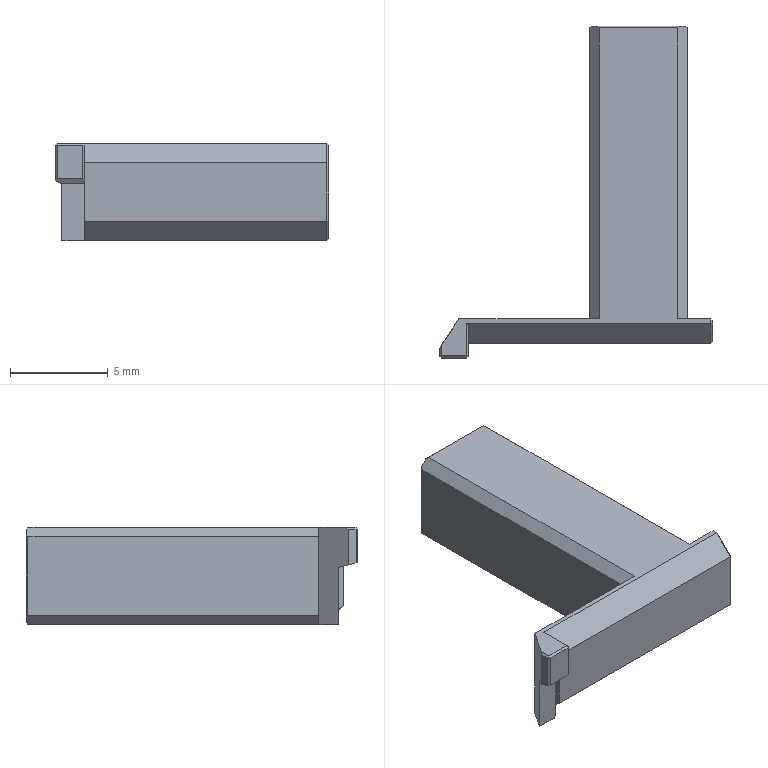Part | 1 solid | 45 faces | box 14 x 17 x 5 mm | volume 429.068 mm3 | plane 41 | cylinder 2 | cone 2 | commonest cylinder face diameters 1.6 x2
STEP:
#1=CARTESIAN_POINT('',(0.,9.8,-0.8));
#2=VERTEX_POINT('',#1);
#3=CARTESIAN_POINT('',(0.,9.8,0.8));
#4=VERTEX_POINT('',#3);
#5=CARTESIAN_POINT('',(0.,9.8,0.));
#6=DIRECTION('',(0.,1.,0.));
#7=DIRECTION('',(0.,0.,1.));
#8=AXIS2_PLACEMENT_3D('',#5,#6,#7);
#9=CIRCLE('',#8,0.8);
#10=EDGE_CURVE('',#2,#4,#9,.T.);
#11=ORIENTED_EDGE('',*,*,#10,.F.);
#12=CARTESIAN_POINT('',(0.,15.,-0.8));
#13=VERTEX_POINT('',#12);
#14=CARTESIAN_POINT('',(0.,15.,-0.8));
#15=DIRECTION('',(0.,1.,0.));
#16=VECTOR('',#15,1000.);
#17=LINE('',#14,#16);
#18=EDGE_CURVE('',#2,#13,#17,.T.);
#19=ORIENTED_EDGE('',*,*,#18,.T.);
#20=CARTESIAN_POINT('',(0.,15.,0.8));
#21=VERTEX_POINT('',#20);
#22=CARTESIAN_POINT('',(0.,15.,0.));
#23=DIRECTION('',(0.,1.,0.));
#24=DIRECTION('',(0.,0.,1.));
#25=AXIS2_PLACEMENT_3D('',#22,#23,#24);
#26=CIRCLE('',#25,0.8);
#27=EDGE_CURVE('',#13,#21,#26,.T.);
#28=ORIENTED_EDGE('',*,*,#27,.T.);
#29=CARTESIAN_POINT('',(0.,15.,0.8));
#30=DIRECTION('',(0.,1.,0.));
#31=VECTOR('',#30,1000.);
#32=LINE('',#29,#31);
#33=EDGE_CURVE('',#4,#21,#32,.T.);
#34=ORIENTED_EDGE('',*,*,#33,.F.);
#35=EDGE_LOOP('',(#11,#19,#28,#34));
#36=FACE_OUTER_BOUND('',#35,.T.);
#37=CARTESIAN_POINT('',(0.,15.,0.));
#38=DIRECTION('',(0.,1.,0.));
#39=DIRECTION('',(0.,0.,1.));
#40=AXIS2_PLACEMENT_3D('',#37,#38,#39);
#41=CYLINDRICAL_SURFACE('',#40,0.8);
#42=ADVANCED_FACE('',(#36),#41,.F.);
#43=CARTESIAN_POINT('',(0.,9.319,0.));
#44=VERTEX_POINT('',#43);
#45=CARTESIAN_POINT('',(0.,9.8,0.8));
#46=DIRECTION('',(0.,0.515,0.8572));
#47=VECTOR('',#46,1000.);
#48=LINE('',#45,#47);
#49=EDGE_CURVE('',#44,#4,#48,.T.);
#50=ORIENTED_EDGE('',*,*,#49,.F.);
#51=CARTESIAN_POINT('',(0.,9.8,-0.8));
#52=DIRECTION('',(0.,0.515,-0.8572));
#53=VECTOR('',#52,1000.);
#54=LINE('',#51,#53);
#55=EDGE_CURVE('',#44,#2,#54,.T.);
#56=ORIENTED_EDGE('',*,*,#55,.T.);
#57=ORIENTED_EDGE('',*,*,#10,.T.);
#58=EDGE_LOOP('',(#50,#56,#57));
#59=FACE_OUTER_BOUND('',#58,.T.);
#60=CARTESIAN_POINT('',(0.,9.8,0.));
#61=DIRECTION('',(0.,1.,0.));
#62=DIRECTION('',(0.,0.,1.));
#63=AXIS2_PLACEMENT_3D('',#60,#61,#62);
#64=CONICAL_SURFACE('',#63,0.8,1.03);
#65=ADVANCED_FACE('',(#59),#64,.F.);
#66=CARTESIAN_POINT('',(-8.7,-1.9,2.4));
#67=VERTEX_POINT('',#66);
#68=CARTESIAN_POINT('',(-8.7,-1.9,0.6751));
#69=VERTEX_POINT('',#68);
#70=CARTESIAN_POINT('',(-8.7,-1.9,-2.5));
#71=DIRECTION('',(0.,0.,-1.));
#72=VECTOR('',#71,1000.);
#73=LINE('',#70,#72);
#74=EDGE_CURVE('',#67,#69,#73,.T.);
#75=ORIENTED_EDGE('',*,*,#74,.T.);
#76=CARTESIAN_POINT('',(-8.7,-1.25,0.501));
#77=VERTEX_POINT('',#76);
#78=CARTESIAN_POINT('',(-8.7,-2.,0.7019));
#79=DIRECTION('',(0.,0.9659,-0.2588));
#80=VECTOR('',#79,1000.);
#81=LINE('',#78,#80);
#82=EDGE_CURVE('',#69,#77,#81,.T.);
#83=ORIENTED_EDGE('',*,*,#82,.T.);
#84=CARTESIAN_POINT('',(-8.7,-1.25,1.5));
#85=VERTEX_POINT('',#84);
#86=CARTESIAN_POINT('',(-8.7,-1.25,-2.5));
#87=DIRECTION('',(0.,0.,1.));
#88=VECTOR('',#87,1000.);
#89=LINE('',#86,#88);
#90=EDGE_CURVE('',#77,#85,#89,.T.);
#91=ORIENTED_EDGE('',*,*,#90,.T.);
#92=CARTESIAN_POINT('',(-8.7,-0.35,2.4));
#93=VERTEX_POINT('',#92);
#94=CARTESIAN_POINT('',(-8.7,-3.625,-0.875));
#95=DIRECTION('',(0.,0.7071,0.7071));
#96=VECTOR('',#95,1000.);
#97=LINE('',#94,#96);
#98=EDGE_CURVE('',#85,#93,#97,.T.);
#99=ORIENTED_EDGE('',*,*,#98,.T.);
#100=CARTESIAN_POINT('',(-8.7,-2.,2.4));
#101=DIRECTION('',(0.,-1.,0.));
#102=VECTOR('',#101,1000.);
#103=LINE('',#100,#102);
#104=EDGE_CURVE('',#93,#67,#103,.T.);
#105=ORIENTED_EDGE('',*,*,#104,.T.);
#106=EDGE_LOOP('',(#75,#83,#91,#99,#105));
#107=FACE_OUTER_BOUND('',#106,.T.);
#108=CARTESIAN_POINT('',(-8.7,-2.,-2.5));
#109=DIRECTION('',(-1.,0.,0.));
#110=DIRECTION('',(0.,0.,1.));
#111=AXIS2_PLACEMENT_3D('',#108,#109,#110);
#112=PLANE('',#111);
#113=ADVANCED_FACE('',(#107),#112,.F.);
#114=CARTESIAN_POINT('',(2.5,14.9,-2.));
#115=VERTEX_POINT('',#114);
#116=CARTESIAN_POINT('',(2.5,14.9,2.));
#117=VERTEX_POINT('',#116);
#118=CARTESIAN_POINT('',(2.5,14.9,2.5));
#119=DIRECTION('',(0.,0.,1.));
#120=VECTOR('',#119,1000.);
#121=LINE('',#118,#120);
#122=EDGE_CURVE('',#115,#117,#121,.T.);
#123=ORIENTED_EDGE('',*,*,#122,.T.);
#124=CARTESIAN_POINT('',(2.5,0.,2.));
#125=VERTEX_POINT('',#124);
#126=CARTESIAN_POINT('',(2.5,15.,2.));
#127=DIRECTION('',(0.,-1.,0.));
#128=VECTOR('',#127,1000.);
#129=LINE('',#126,#128);
#130=EDGE_CURVE('',#117,#125,#129,.T.);
#131=ORIENTED_EDGE('',*,*,#130,.T.);
#132=CARTESIAN_POINT('',(2.5,0.,-2.));
#133=VERTEX_POINT('',#132);
#134=CARTESIAN_POINT('',(2.5,0.,2.5));
#135=DIRECTION('',(0.,0.,-1.));
#136=VECTOR('',#135,1000.);
#137=LINE('',#134,#136);
#138=EDGE_CURVE('',#125,#133,#137,.T.);
#139=ORIENTED_EDGE('',*,*,#138,.T.);
#140=CARTESIAN_POINT('',(2.5,15.,-2.));
#141=DIRECTION('',(0.,1.,0.));
#142=VECTOR('',#141,1000.);
#143=LINE('',#140,#142);
#144=EDGE_CURVE('',#133,#115,#143,.T.);
#145=ORIENTED_EDGE('',*,*,#144,.T.);
#146=EDGE_LOOP('',(#123,#131,#139,#145));
#147=FACE_OUTER_BOUND('',#146,.T.);
#148=CARTESIAN_POINT('',(2.5,15.,2.5));
#149=DIRECTION('',(-1.,0.,0.));
#150=DIRECTION('',(0.,0.,1.));
#151=AXIS2_PLACEMENT_3D('',#148,#149,#150);
#152=PLANE('',#151);
#153=ADVANCED_FACE('',(#147),#152,.F.);
#154=CARTESIAN_POINT('',(-8.8,-0.25,-2.5));
#155=VERTEX_POINT('',#154);
#156=CARTESIAN_POINT('',(-8.8,-1.,-2.5));
#157=VERTEX_POINT('',#156);
#158=CARTESIAN_POINT('',(-8.8,15.,-2.5));
#159=DIRECTION('',(0.,-1.,0.));
#160=VECTOR('',#159,1000.);
#161=LINE('',#158,#160);
#162=EDGE_CURVE('',#155,#157,#161,.T.);
#163=ORIENTED_EDGE('',*,*,#162,.T.);
#164=CARTESIAN_POINT('',(-9.867,-1.,-2.5));
#165=VERTEX_POINT('',#164);
#166=CARTESIAN_POINT('',(-10.2,-1.,-2.5));
#167=DIRECTION('',(1.,0.,0.));
#168=VECTOR('',#167,1000.);
#169=LINE('',#166,#168);
#170=EDGE_CURVE('',#165,#157,#169,.T.);
#171=ORIENTED_EDGE('',*,*,#170,.F.);
#172=CARTESIAN_POINT('',(-9.2,0.,-2.5));
#173=VERTEX_POINT('',#172);
#174=CARTESIAN_POINT('',(-0.2154,13.477,-2.5));
#175=DIRECTION('',(0.5547,0.8321,0.));
#176=VECTOR('',#175,1000.);
#177=LINE('',#174,#176);
#178=EDGE_CURVE('',#165,#173,#177,.T.);
#179=ORIENTED_EDGE('',*,*,#178,.T.);
#180=CARTESIAN_POINT('',(-2.,0.,-2.5));
#181=VERTEX_POINT('',#180);
#182=CARTESIAN_POINT('',(3.8,0.,-2.5));
#183=DIRECTION('',(1.,0.,0.));
#184=VECTOR('',#183,1000.);
#185=LINE('',#182,#184);
#186=EDGE_CURVE('',#173,#181,#185,.T.);
#187=ORIENTED_EDGE('',*,*,#186,.T.);
#188=CARTESIAN_POINT('',(-2.,14.9,-2.5));
#189=VERTEX_POINT('',#188);
#190=CARTESIAN_POINT('',(-2.,15.,-2.5));
#191=DIRECTION('',(0.,1.,0.));
#192=VECTOR('',#191,1000.);
#193=LINE('',#190,#192);
#194=EDGE_CURVE('',#181,#189,#193,.T.);
#195=ORIENTED_EDGE('',*,*,#194,.T.);
#196=CARTESIAN_POINT('',(2.,14.9,-2.5));
#197=VERTEX_POINT('',#196);
#198=CARTESIAN_POINT('',(-2.5,14.9,-2.5));
#199=DIRECTION('',(1.,0.,0.));
#200=VECTOR('',#199,1000.);
#201=LINE('',#198,#200);
#202=EDGE_CURVE('',#189,#197,#201,.T.);
#203=ORIENTED_EDGE('',*,*,#202,.T.);
#204=CARTESIAN_POINT('',(2.,0.,-2.5));
#205=VERTEX_POINT('',#204);
#206=CARTESIAN_POINT('',(2.,15.,-2.5));
#207=DIRECTION('',(0.,-1.,0.));
#208=VECTOR('',#207,1000.);
#209=LINE('',#206,#208);
#210=EDGE_CURVE('',#197,#205,#209,.T.);
#211=ORIENTED_EDGE('',*,*,#210,.T.);
#212=CARTESIAN_POINT('',(3.7,0.,-2.5));
#213=VERTEX_POINT('',#212);
#214=CARTESIAN_POINT('',(3.8,0.,-2.5));
#215=DIRECTION('',(1.,0.,0.));
#216=VECTOR('',#215,1000.);
#217=LINE('',#214,#216);
#218=EDGE_CURVE('',#205,#213,#217,.T.);
#219=ORIENTED_EDGE('',*,*,#218,.T.);
#220=CARTESIAN_POINT('',(3.7,-0.25,-2.5));
#221=VERTEX_POINT('',#220);
#222=CARTESIAN_POINT('',(3.7,15.,-2.5));
#223=DIRECTION('',(0.,-1.,0.));
#224=VECTOR('',#223,1000.);
#225=LINE('',#222,#224);
#226=EDGE_CURVE('',#213,#221,#225,.T.);
#227=ORIENTED_EDGE('',*,*,#226,.T.);
#228=CARTESIAN_POINT('',(-2.5,-0.25,-2.5));
#229=DIRECTION('',(-1.,0.,0.));
#230=VECTOR('',#229,1000.);
#231=LINE('',#228,#230);
#232=EDGE_CURVE('',#221,#155,#231,.T.);
#233=ORIENTED_EDGE('',*,*,#232,.T.);
#234=EDGE_LOOP('',(#163,#171,#179,#187,#195,#203,#211,#219,#227,#233));
#235=FACE_OUTER_BOUND('',#234,.T.);
#236=CARTESIAN_POINT('',(-2.5,15.,-2.5));
#237=DIRECTION('',(0.,0.,1.));
#238=DIRECTION('',(1.,0.,0.));
#239=AXIS2_PLACEMENT_3D('',#236,#237,#238);
#240=PLANE('',#239);
#241=ADVANCED_FACE('',(#235),#240,.F.);
#242=CARTESIAN_POINT('',(-2.5,0.,-2.));
#243=VERTEX_POINT('',#242);
#244=CARTESIAN_POINT('',(-2.5,0.,2.));
#245=VERTEX_POINT('',#244);
#246=CARTESIAN_POINT('',(-2.5,0.,2.5));
#247=DIRECTION('',(0.,0.,1.));
#248=VECTOR('',#247,1000.);
#249=LINE('',#246,#248);
#250=EDGE_CURVE('',#243,#245,#249,.T.);
#251=ORIENTED_EDGE('',*,*,#250,.T.);
#252=CARTESIAN_POINT('',(-2.5,14.9,2.));
#253=VERTEX_POINT('',#252);
#254=CARTESIAN_POINT('',(-2.5,15.,2.));
#255=DIRECTION('',(0.,1.,0.));
#256=VECTOR('',#255,1000.);
#257=LINE('',#254,#256);
#258=EDGE_CURVE('',#245,#253,#257,.T.);
#259=ORIENTED_EDGE('',*,*,#258,.T.);
#260=CARTESIAN_POINT('',(-2.5,14.9,-2.));
#261=VERTEX_POINT('',#260);
#262=CARTESIAN_POINT('',(-2.5,14.9,2.5));
#263=DIRECTION('',(0.,0.,-1.));
#264=VECTOR('',#263,1000.);
#265=LINE('',#262,#264);
#266=EDGE_CURVE('',#253,#261,#265,.T.);
#267=ORIENTED_EDGE('',*,*,#266,.T.);
#268=CARTESIAN_POINT('',(-2.5,15.,-2.));
#269=DIRECTION('',(0.,-1.,0.));
#270=VECTOR('',#269,1000.);
#271=LINE('',#268,#270);
#272=EDGE_CURVE('',#261,#243,#271,.T.);
#273=ORIENTED_EDGE('',*,*,#272,.T.);
#274=EDGE_LOOP('',(#251,#259,#267,#273));
#275=FACE_OUTER_BOUND('',#274,.T.);
#276=CARTESIAN_POINT('',(-2.5,15.,2.5));
#277=DIRECTION('',(1.,0.,0.));
#278=DIRECTION('',(0.,0.,-1.));
#279=AXIS2_PLACEMENT_3D('',#276,#277,#278);
#280=PLANE('',#279);
#281=ADVANCED_FACE('',(#275),#280,.F.);
#282=CARTESIAN_POINT('',(-2.,0.,2.5));
#283=VERTEX_POINT('',#282);
#284=CARTESIAN_POINT('',(-9.2,0.,2.5));
#285=VERTEX_POINT('',#284);
#286=CARTESIAN_POINT('',(3.8,0.,2.5));
#287=DIRECTION('',(-1.,0.,0.));
#288=VECTOR('',#287,1000.);
#289=LINE('',#286,#288);
#290=EDGE_CURVE('',#283,#285,#289,.T.);
#291=ORIENTED_EDGE('',*,*,#290,.T.);
#292=CARTESIAN_POINT('',(-10.1,-1.35,2.5));
#293=VERTEX_POINT('',#292);
#294=CARTESIAN_POINT('',(-10.2,-1.5,2.5));
#295=DIRECTION('',(0.5547,0.8321,0.));
#296=VECTOR('',#295,1000.);
#297=LINE('',#294,#296);
#298=EDGE_CURVE('',#293,#285,#297,.T.);
#299=ORIENTED_EDGE('',*,*,#298,.F.);
#300=CARTESIAN_POINT('',(-10.1,-1.9,2.5));
#301=VERTEX_POINT('',#300);
#302=CARTESIAN_POINT('',(-10.1,15.,2.5));
#303=DIRECTION('',(0.,-1.,0.));
#304=VECTOR('',#303,1000.);
#305=LINE('',#302,#304);
#306=EDGE_CURVE('',#293,#301,#305,.T.);
#307=ORIENTED_EDGE('',*,*,#306,.T.);
#308=CARTESIAN_POINT('',(-8.8,-1.9,2.5));
#309=VERTEX_POINT('',#308);
#310=CARTESIAN_POINT('',(-2.5,-1.9,2.5));
#311=DIRECTION('',(1.,0.,0.));
#312=VECTOR('',#311,1000.);
#313=LINE('',#310,#312);
#314=EDGE_CURVE('',#301,#309,#313,.T.);
#315=ORIENTED_EDGE('',*,*,#314,.T.);
#316=CARTESIAN_POINT('',(-8.8,-0.25,2.5));
#317=VERTEX_POINT('',#316);
#318=CARTESIAN_POINT('',(-8.8,15.,2.5));
#319=DIRECTION('',(0.,1.,0.));
#320=VECTOR('',#319,1000.);
#321=LINE('',#318,#320);
#322=EDGE_CURVE('',#309,#317,#321,.T.);
#323=ORIENTED_EDGE('',*,*,#322,.T.);
#324=CARTESIAN_POINT('',(3.7,-0.25,2.5));
#325=VERTEX_POINT('',#324);
#326=CARTESIAN_POINT('',(-2.5,-0.25,2.5));
#327=DIRECTION('',(1.,0.,0.));
#328=VECTOR('',#327,1000.);
#329=LINE('',#326,#328);
#330=EDGE_CURVE('',#317,#325,#329,.T.);
#331=ORIENTED_EDGE('',*,*,#330,.T.);
#332=CARTESIAN_POINT('',(3.7,0.,2.5));
#333=VERTEX_POINT('',#332);
#334=CARTESIAN_POINT('',(3.7,15.,2.5));
#335=DIRECTION('',(0.,1.,0.));
#336=VECTOR('',#335,1000.);
#337=LINE('',#334,#336);
#338=EDGE_CURVE('',#325,#333,#337,.T.);
#339=ORIENTED_EDGE('',*,*,#338,.T.);
#340=CARTESIAN_POINT('',(2.,0.,2.5));
#341=VERTEX_POINT('',#340);
#342=CARTESIAN_POINT('',(3.8,0.,2.5));
#343=DIRECTION('',(-1.,0.,0.));
#344=VECTOR('',#343,1000.);
#345=LINE('',#342,#344);
#346=EDGE_CURVE('',#333,#341,#345,.T.);
#347=ORIENTED_EDGE('',*,*,#346,.T.);
#348=CARTESIAN_POINT('',(2.,14.9,2.5));
#349=VERTEX_POINT('',#348);
#350=CARTESIAN_POINT('',(2.,15.,2.5));
#351=DIRECTION('',(0.,1.,0.));
#352=VECTOR('',#351,1000.);
#353=LINE('',#350,#352);
#354=EDGE_CURVE('',#341,#349,#353,.T.);
#355=ORIENTED_EDGE('',*,*,#354,.T.);
#356=CARTESIAN_POINT('',(-2.,14.9,2.5));
#357=VERTEX_POINT('',#356);
#358=CARTESIAN_POINT('',(-2.5,14.9,2.5));
#359=DIRECTION('',(-1.,0.,0.));
#360=VECTOR('',#359,1000.);
#361=LINE('',#358,#360);
#362=EDGE_CURVE('',#349,#357,#361,.T.);
#363=ORIENTED_EDGE('',*,*,#362,.T.);
#364=CARTESIAN_POINT('',(-2.,15.,2.5));
#365=DIRECTION('',(0.,-1.,0.));
#366=VECTOR('',#365,1000.);
#367=LINE('',#364,#366);
#368=EDGE_CURVE('',#357,#283,#367,.T.);
#369=ORIENTED_EDGE('',*,*,#368,.T.);
#370=EDGE_LOOP('',(#291,#299,#307,#315,#323,#331,#339,#347,#355,#363,#369));
#371=FACE_OUTER_BOUND('',#370,.T.);
#372=CARTESIAN_POINT('',(-2.5,15.,2.5));
#373=DIRECTION('',(0.,0.,-1.));
#374=DIRECTION('',(-1.,0.,0.));
#375=AXIS2_PLACEMENT_3D('',#372,#373,#374);
#376=PLANE('',#375);
#377=ADVANCED_FACE('',(#371),#376,.F.);
#378=CARTESIAN_POINT('',(-2.4,15.,-2.1));
#379=VERTEX_POINT('',#378);
#380=CARTESIAN_POINT('',(-2.4,15.,2.1));
#381=VERTEX_POINT('',#380);
#382=CARTESIAN_POINT('',(-2.4,15.,0.));
#383=DIRECTION('',(0.,0.,1.));
#384=VECTOR('',#383,1000.);
#385=LINE('',#382,#384);
#386=EDGE_CURVE('',#379,#381,#385,.T.);
#387=ORIENTED_EDGE('',*,*,#386,.T.);
#388=CARTESIAN_POINT('',(-2.1,15.,2.4));
#389=VERTEX_POINT('',#388);
#390=CARTESIAN_POINT('',(-2.,15.,2.5));
#391=DIRECTION('',(0.7071,0.,0.7071));
#392=VECTOR('',#391,1000.);
#393=LINE('',#390,#392);
#394=EDGE_CURVE('',#381,#389,#393,.T.);
#395=ORIENTED_EDGE('',*,*,#394,.T.);
#396=CARTESIAN_POINT('',(2.1,15.,2.4));
#397=VERTEX_POINT('',#396);
#398=CARTESIAN_POINT('',(0.,15.,2.4));
#399=DIRECTION('',(1.,0.,0.));
#400=VECTOR('',#399,1000.);
#401=LINE('',#398,#400);
#402=EDGE_CURVE('',#389,#397,#401,.T.);
#403=ORIENTED_EDGE('',*,*,#402,.T.);
#404=CARTESIAN_POINT('',(2.4,15.,2.1));
#405=VERTEX_POINT('',#404);
#406=CARTESIAN_POINT('',(2.5,15.,2.));
#407=DIRECTION('',(0.7071,0.,-0.7071));
#408=VECTOR('',#407,1000.);
#409=LINE('',#406,#408);
#410=EDGE_CURVE('',#397,#405,#409,.T.);
#411=ORIENTED_EDGE('',*,*,#410,.T.);
#412=CARTESIAN_POINT('',(2.4,15.,-2.1));
#413=VERTEX_POINT('',#412);
#414=CARTESIAN_POINT('',(2.4,15.,0.));
#415=DIRECTION('',(0.,0.,-1.));
#416=VECTOR('',#415,1000.);
#417=LINE('',#414,#416);
#418=EDGE_CURVE('',#405,#413,#417,.T.);
#419=ORIENTED_EDGE('',*,*,#418,.T.);
#420=CARTESIAN_POINT('',(2.1,15.,-2.4));
#421=VERTEX_POINT('',#420);
#422=CARTESIAN_POINT('',(2.,15.,-2.5));
#423=DIRECTION('',(-0.7071,0.,-0.7071));
#424=VECTOR('',#423,1000.);
#425=LINE('',#422,#424);
#426=EDGE_CURVE('',#413,#421,#425,.T.);
#427=ORIENTED_EDGE('',*,*,#426,.T.);
#428=CARTESIAN_POINT('',(-2.1,15.,-2.4));
#429=VERTEX_POINT('',#428);
#430=CARTESIAN_POINT('',(0.,15.,-2.4));
#431=DIRECTION('',(-1.,0.,0.));
#432=VECTOR('',#431,1000.);
#433=LINE('',#430,#432);
#434=EDGE_CURVE('',#421,#429,#433,.T.);
#435=ORIENTED_EDGE('',*,*,#434,.T.);
#436=CARTESIAN_POINT('',(-2.5,15.,-2.));
#437=DIRECTION('',(-0.7071,0.,0.7071));
#438=VECTOR('',#437,1000.);
#439=LINE('',#436,#438);
#440=EDGE_CURVE('',#429,#379,#439,.T.);
#441=ORIENTED_EDGE('',*,*,#440,.T.);
#442=EDGE_LOOP('',(#387,#395,#403,#411,#419,#427,#435,#441));
#443=FACE_OUTER_BOUND('',#442,.T.);
#444=CARTESIAN_POINT('',(0.,15.,0.));
#445=DIRECTION('',(0.,1.,0.));
#446=DIRECTION('',(0.,0.,1.));
#447=AXIS2_PLACEMENT_3D('',#444,#445,#446);
#448=CIRCLE('',#447,0.8);
#449=EDGE_CURVE('',#21,#13,#448,.T.);
#450=ORIENTED_EDGE('',*,*,#449,.F.);
#451=ORIENTED_EDGE('',*,*,#27,.F.);
#452=EDGE_LOOP('',(#450,#451));
#453=FACE_BOUND('',#452,.T.);
#454=CARTESIAN_POINT('',(0.,15.,0.));
#455=DIRECTION('',(0.,-1.,0.));
#456=DIRECTION('',(0.,0.,-1.));
#457=AXIS2_PLACEMENT_3D('',#454,#455,#456);
#458=PLANE('',#457);
#459=ADVANCED_FACE('',(#443,#453),#458,.F.);
#460=ORIENTED_EDGE('',*,*,#55,.F.);
#461=ORIENTED_EDGE('',*,*,#49,.T.);
#462=CARTESIAN_POINT('',(0.,9.8,0.));
#463=DIRECTION('',(0.,1.,0.));
#464=DIRECTION('',(0.,0.,1.));
#465=AXIS2_PLACEMENT_3D('',#462,#463,#464);
#466=CIRCLE('',#465,0.8);
#467=EDGE_CURVE('',#4,#2,#466,.T.);
#468=ORIENTED_EDGE('',*,*,#467,.T.);
#469=EDGE_LOOP('',(#460,#461,#468));
#470=FACE_OUTER_BOUND('',#469,.T.);
#471=CARTESIAN_POINT('',(0.,9.8,0.));
#472=DIRECTION('',(0.,1.,0.));
#473=DIRECTION('',(0.,0.,1.));
#474=AXIS2_PLACEMENT_3D('',#471,#472,#473);
#475=CONICAL_SURFACE('',#474,0.8,1.03);
#476=ADVANCED_FACE('',(#470),#475,.F.);
#477=ORIENTED_EDGE('',*,*,#18,.F.);
#478=ORIENTED_EDGE('',*,*,#467,.F.);
#479=ORIENTED_EDGE('',*,*,#33,.T.);
#480=ORIENTED_EDGE('',*,*,#449,.T.);
#481=EDGE_LOOP('',(#477,#478,#479,#480));
#482=FACE_OUTER_BOUND('',#481,.T.);
#483=CARTESIAN_POINT('',(0.,15.,0.));
#484=DIRECTION('',(0.,1.,0.));
#485=DIRECTION('',(0.,0.,1.));
#486=AXIS2_PLACEMENT_3D('',#483,#484,#485);
#487=CYLINDRICAL_SURFACE('',#486,0.8);
#488=ADVANCED_FACE('',(#482),#487,.F.);
#489=ORIENTED_EDGE('',*,*,#346,.F.);
#490=CARTESIAN_POINT('',(3.7,0.,-2.5));
#491=DIRECTION('',(0.,0.,-1.));
#492=VECTOR('',#491,1000.);
#493=LINE('',#490,#492);
#494=EDGE_CURVE('',#333,#213,#493,.T.);
#495=ORIENTED_EDGE('',*,*,#494,.T.);
#496=ORIENTED_EDGE('',*,*,#218,.F.);
#497=CARTESIAN_POINT('',(2.,0.,-2.5));
#498=DIRECTION('',(0.7071,0.,0.7071));
#499=VECTOR('',#498,1000.);
#500=LINE('',#497,#499);
#501=EDGE_CURVE('',#205,#133,#500,.T.);
#502=ORIENTED_EDGE('',*,*,#501,.T.);
#503=ORIENTED_EDGE('',*,*,#138,.F.);
#504=CARTESIAN_POINT('',(2.5,0.,2.));
#505=DIRECTION('',(-0.7071,0.,0.7071));
#506=VECTOR('',#505,1000.);
#507=LINE('',#504,#506);
#508=EDGE_CURVE('',#125,#341,#507,.T.);
#509=ORIENTED_EDGE('',*,*,#508,.T.);
#510=EDGE_LOOP('',(#489,#495,#496,#502,#503,#509));
#511=FACE_OUTER_BOUND('',#510,.T.);
#512=CARTESIAN_POINT('',(0.,0.,0.));
#513=DIRECTION('',(0.,1.,0.));
#514=DIRECTION('',(0.,0.,1.));
#515=AXIS2_PLACEMENT_3D('',#512,#513,#514);
#516=PLANE('',#515);
#517=ADVANCED_FACE('',(#511),#516,.T.);
#518=CARTESIAN_POINT('',(-9.2,0.,-7.5));
#519=DIRECTION('',(0.,0.,1.));
#520=VECTOR('',#519,1000.);
#521=LINE('',#518,#520);
#522=EDGE_CURVE('',#173,#285,#521,.T.);
#523=ORIENTED_EDGE('',*,*,#522,.T.);
#524=ORIENTED_EDGE('',*,*,#290,.F.);
#525=CARTESIAN_POINT('',(-2.,0.,2.5));
#526=DIRECTION('',(-0.7071,0.,-0.7071));
#527=VECTOR('',#526,1000.);
#528=LINE('',#525,#527);
#529=EDGE_CURVE('',#283,#245,#528,.T.);
#530=ORIENTED_EDGE('',*,*,#529,.T.);
#531=ORIENTED_EDGE('',*,*,#250,.F.);
#532=CARTESIAN_POINT('',(-2.5,0.,-2.));
#533=DIRECTION('',(0.7071,0.,-0.7071));
#534=VECTOR('',#533,1000.);
#535=LINE('',#532,#534);
#536=EDGE_CURVE('',#243,#181,#535,.T.);
#537=ORIENTED_EDGE('',*,*,#536,.T.);
#538=ORIENTED_EDGE('',*,*,#186,.F.);
#539=EDGE_LOOP('',(#523,#524,#530,#531,#537,#538));
#540=FACE_OUTER_BOUND('',#539,.T.);
#541=CARTESIAN_POINT('',(0.,0.,0.));
#542=DIRECTION('',(0.,1.,0.));
#543=DIRECTION('',(0.,0.,1.));
#544=AXIS2_PLACEMENT_3D('',#541,#542,#543);
#545=PLANE('',#544);
#546=ADVANCED_FACE('',(#540),#545,.T.);
#547=CARTESIAN_POINT('',(3.8,-0.1,2.4));
#548=VERTEX_POINT('',#547);
#549=CARTESIAN_POINT('',(3.8,-0.2086,2.4));
#550=VERTEX_POINT('',#549);
#551=CARTESIAN_POINT('',(3.8,-2.,2.4));
#552=DIRECTION('',(0.,-1.,0.));
#553=VECTOR('',#552,1000.);
#554=LINE('',#551,#553);
#555=EDGE_CURVE('',#548,#550,#554,.T.);
#556=ORIENTED_EDGE('',*,*,#555,.T.);
#557=CARTESIAN_POINT('',(3.8,-1.15,1.459));
#558=VERTEX_POINT('',#557);
#559=CARTESIAN_POINT('',(3.8,-1.179,1.429));
#560=DIRECTION('',(0.,-0.7071,-0.7071));
#561=VECTOR('',#560,1000.);
#562=LINE('',#559,#561);
#563=EDGE_CURVE('',#550,#558,#562,.T.);
#564=ORIENTED_EDGE('',*,*,#563,.T.);
#565=CARTESIAN_POINT('',(3.8,-1.15,-1.459));
#566=VERTEX_POINT('',#565);
#567=CARTESIAN_POINT('',(3.8,-1.15,2.5));
#568=DIRECTION('',(0.,0.,-1.));
#569=VECTOR('',#568,1000.);
#570=LINE('',#567,#569);
#571=EDGE_CURVE('',#558,#566,#570,.T.);
#572=ORIENTED_EDGE('',*,*,#571,.T.);
#573=CARTESIAN_POINT('',(3.8,-0.2086,-2.4));
#574=VERTEX_POINT('',#573);
#575=CARTESIAN_POINT('',(3.8,-0.1793,-2.429));
#576=DIRECTION('',(0.,0.7071,-0.7071));
#577=VECTOR('',#576,1000.);
#578=LINE('',#575,#577);
#579=EDGE_CURVE('',#566,#574,#578,.T.);
#580=ORIENTED_EDGE('',*,*,#579,.T.);
#581=CARTESIAN_POINT('',(3.8,-0.1,-2.4));
#582=VERTEX_POINT('',#581);
#583=CARTESIAN_POINT('',(3.8,-2.,-2.4));
#584=DIRECTION('',(0.,1.,0.));
#585=VECTOR('',#584,1000.);
#586=LINE('',#583,#585);
#587=EDGE_CURVE('',#574,#582,#586,.T.);
#588=ORIENTED_EDGE('',*,*,#587,.T.);
#589=CARTESIAN_POINT('',(3.8,-0.1,2.5));
#590=DIRECTION('',(0.,0.,1.));
#591=VECTOR('',#590,1000.);
#592=LINE('',#589,#591);
#593=EDGE_CURVE('',#582,#548,#592,.T.);
#594=ORIENTED_EDGE('',*,*,#593,.T.);
#595=EDGE_LOOP('',(#556,#564,#572,#580,#588,#594));
#596=FACE_OUTER_BOUND('',#595,.T.);
#597=CARTESIAN_POINT('',(3.8,-2.,2.5));
#598=DIRECTION('',(-1.,0.,0.));
#599=DIRECTION('',(0.,0.,1.));
#600=AXIS2_PLACEMENT_3D('',#597,#598,#599);
#601=PLANE('',#600);
#602=ADVANCED_FACE('',(#596),#601,.F.);
#603=CARTESIAN_POINT('',(-10.2,-1.5,0.5679));
#604=VERTEX_POINT('',#603);
#605=CARTESIAN_POINT('',(-10.2,-1.5,2.4));
#606=VERTEX_POINT('',#605);
#607=CARTESIAN_POINT('',(-10.2,-1.5,-7.5));
#608=DIRECTION('',(0.,0.,1.));
#609=VECTOR('',#608,1000.);
#610=LINE('',#607,#609);
#611=EDGE_CURVE('',#604,#606,#610,.T.);
#612=ORIENTED_EDGE('',*,*,#611,.F.);
#613=CARTESIAN_POINT('',(-10.2,-1.9,0.6751));
#614=VERTEX_POINT('',#613);
#615=CARTESIAN_POINT('',(-10.2,-2.,0.7019));
#616=DIRECTION('',(0.,-0.9659,0.2588));
#617=VECTOR('',#616,1000.);
#618=LINE('',#615,#617);
#619=EDGE_CURVE('',#604,#614,#618,.T.);
#620=ORIENTED_EDGE('',*,*,#619,.T.);
#621=CARTESIAN_POINT('',(-10.2,-1.9,2.4));
#622=VERTEX_POINT('',#621);
#623=CARTESIAN_POINT('',(-10.2,-1.9,2.5));
#624=DIRECTION('',(0.,0.,1.));
#625=VECTOR('',#624,1000.);
#626=LINE('',#623,#625);
#627=EDGE_CURVE('',#614,#622,#626,.T.);
#628=ORIENTED_EDGE('',*,*,#627,.T.);
#629=CARTESIAN_POINT('',(-10.2,-2.,2.4));
#630=DIRECTION('',(0.,1.,0.));
#631=VECTOR('',#630,1000.);
#632=LINE('',#629,#631);
#633=EDGE_CURVE('',#622,#606,#632,.T.);
#634=ORIENTED_EDGE('',*,*,#633,.T.);
#635=EDGE_LOOP('',(#612,#620,#628,#634));
#636=FACE_OUTER_BOUND('',#635,.T.);
#637=CARTESIAN_POINT('',(-10.2,-2.,2.5));
#638=DIRECTION('',(1.,0.,0.));
#639=DIRECTION('',(0.,0.,-1.));
#640=AXIS2_PLACEMENT_3D('',#637,#638,#639);
#641=PLANE('',#640);
#642=ADVANCED_FACE('',(#636),#641,.F.);
#643=CARTESIAN_POINT('',(-10.1,-2.,2.4));
#644=VERTEX_POINT('',#643);
#645=CARTESIAN_POINT('',(-10.1,-2.,0.7019));
#646=VERTEX_POINT('',#645);
#647=CARTESIAN_POINT('',(-10.1,-2.,0.));
#648=DIRECTION('',(0.,0.,-1.));
#649=VECTOR('',#648,1000.);
#650=LINE('',#647,#649);
#651=EDGE_CURVE('',#644,#646,#650,.T.);
#652=ORIENTED_EDGE('',*,*,#651,.T.);
#653=CARTESIAN_POINT('',(-8.8,-2.,0.7019));
#654=VERTEX_POINT('',#653);
#655=CARTESIAN_POINT('',(0.,-2.,0.7019));
#656=DIRECTION('',(1.,0.,0.));
#657=VECTOR('',#656,1000.);
#658=LINE('',#655,#657);
#659=EDGE_CURVE('',#646,#654,#658,.T.);
#660=ORIENTED_EDGE('',*,*,#659,.T.);
#661=CARTESIAN_POINT('',(-8.8,-2.,2.4));
#662=VERTEX_POINT('',#661);
#663=CARTESIAN_POINT('',(-8.8,-2.,0.));
#664=DIRECTION('',(0.,0.,1.));
#665=VECTOR('',#664,1000.);
#666=LINE('',#663,#665);
#667=EDGE_CURVE('',#654,#662,#666,.T.);
#668=ORIENTED_EDGE('',*,*,#667,.T.);
#669=CARTESIAN_POINT('',(0.,-2.,2.4));
#670=DIRECTION('',(-1.,0.,0.));
#671=VECTOR('',#670,1000.);
#672=LINE('',#669,#671);
#673=EDGE_CURVE('',#662,#644,#672,.T.);
#674=ORIENTED_EDGE('',*,*,#673,.T.);
#675=EDGE_LOOP('',(#652,#660,#668,#674));
#676=FACE_OUTER_BOUND('',#675,.T.);
#677=CARTESIAN_POINT('',(0.,-2.,0.));
#678=DIRECTION('',(0.,1.,0.));
#679=DIRECTION('',(0.,0.,1.));
#680=AXIS2_PLACEMENT_3D('',#677,#678,#679);
#681=PLANE('',#680);
#682=ADVANCED_FACE('',(#676),#681,.F.);
#683=CARTESIAN_POINT('',(-8.7,-0.35,-2.4));
#684=VERTEX_POINT('',#683);
#685=CARTESIAN_POINT('',(-8.7,-1.,-1.75));
#686=VERTEX_POINT('',#685);
#687=CARTESIAN_POINT('',(-8.7,-1.125,-1.625));
#688=DIRECTION('',(0.,-0.7071,0.7071));
#689=VECTOR('',#688,1000.);
#690=LINE('',#687,#689);
#691=EDGE_CURVE('',#684,#686,#690,.T.);
#692=ORIENTED_EDGE('',*,*,#691,.T.);
#693=CARTESIAN_POINT('',(-8.7,-1.,-2.4));
#694=VERTEX_POINT('',#693);
#695=CARTESIAN_POINT('',(-8.7,-1.,0.3));
#696=DIRECTION('',(0.,0.,1.));
#697=VECTOR('',#696,1000.);
#698=LINE('',#695,#697);
#699=EDGE_CURVE('',#694,#686,#698,.T.);
#700=ORIENTED_EDGE('',*,*,#699,.F.);
#701=CARTESIAN_POINT('',(-8.7,-2.,-2.4));
#702=DIRECTION('',(0.,1.,0.));
#703=VECTOR('',#702,1000.);
#704=LINE('',#701,#703);
#705=EDGE_CURVE('',#694,#684,#704,.T.);
#706=ORIENTED_EDGE('',*,*,#705,.T.);
#707=EDGE_LOOP('',(#692,#700,#706));
#708=FACE_OUTER_BOUND('',#707,.T.);
#709=CARTESIAN_POINT('',(-8.7,-2.,-2.5));
#710=DIRECTION('',(-1.,0.,0.));
#711=DIRECTION('',(0.,0.,1.));
#712=AXIS2_PLACEMENT_3D('',#709,#710,#711);
#713=PLANE('',#712);
#714=ADVANCED_FACE('',(#708),#713,.F.);
#715=CARTESIAN_POINT('',(-8.7,-1.25,-1.5));
#716=VERTEX_POINT('',#715);
#717=CARTESIAN_POINT('',(3.7,-1.25,-1.5));
#718=VERTEX_POINT('',#717);
#719=CARTESIAN_POINT('',(3.8,-1.25,-1.5));
#720=DIRECTION('',(1.,0.,0.));
#721=VECTOR('',#720,1000.);
#722=LINE('',#719,#721);
#723=EDGE_CURVE('',#716,#718,#722,.T.);
#724=ORIENTED_EDGE('',*,*,#723,.T.);
#725=CARTESIAN_POINT('',(3.7,-1.25,1.5));
#726=VERTEX_POINT('',#725);
#727=CARTESIAN_POINT('',(3.7,-1.25,-2.5));
#728=DIRECTION('',(0.,0.,1.));
#729=VECTOR('',#728,1000.);
#730=LINE('',#727,#729);
#731=EDGE_CURVE('',#718,#726,#730,.T.);
#732=ORIENTED_EDGE('',*,*,#731,.T.);
#733=CARTESIAN_POINT('',(3.8,-1.25,1.5));
#734=DIRECTION('',(-1.,0.,0.));
#735=VECTOR('',#734,1000.);
#736=LINE('',#733,#735);
#737=EDGE_CURVE('',#726,#85,#736,.T.);
#738=ORIENTED_EDGE('',*,*,#737,.T.);
#739=ORIENTED_EDGE('',*,*,#90,.F.);
#740=CARTESIAN_POINT('',(-8.7,-1.25,-2.5));
#741=DIRECTION('',(0.,0.,1.));
#742=VECTOR('',#741,1000.);
#743=LINE('',#740,#742);
#744=EDGE_CURVE('',#716,#77,#743,.T.);
#745=ORIENTED_EDGE('',*,*,#744,.F.);
#746=EDGE_LOOP('',(#724,#732,#738,#739,#745));
#747=FACE_OUTER_BOUND('',#746,.T.);
#748=CARTESIAN_POINT('',(3.8,-1.25,-2.5));
#749=DIRECTION('',(0.,1.,0.));
#750=DIRECTION('',(-1.,0.,0.));
#751=AXIS2_PLACEMENT_3D('',#748,#749,#750);
#752=PLANE('',#751);
#753=ADVANCED_FACE('',(#747),#752,.F.);
#754=ORIENTED_EDGE('',*,*,#232,.F.);
#755=CARTESIAN_POINT('',(3.7,-1.25,-1.5));
#756=DIRECTION('',(0.,-0.7071,0.7071));
#757=VECTOR('',#756,1000.);
#758=LINE('',#755,#757);
#759=EDGE_CURVE('',#221,#718,#758,.T.);
#760=ORIENTED_EDGE('',*,*,#759,.T.);
#761=ORIENTED_EDGE('',*,*,#723,.F.);
#762=CARTESIAN_POINT('',(-8.7,-0.25,-2.5));
#763=DIRECTION('',(0.,0.7071,-0.7071));
#764=VECTOR('',#763,1000.);
#765=LINE('',#762,#764);
#766=EDGE_CURVE('',#716,#686,#765,.T.);
#767=ORIENTED_EDGE('',*,*,#766,.T.);
#768=ORIENTED_EDGE('',*,*,#691,.F.);
#769=CARTESIAN_POINT('',(-13.883,4.833,-7.583));
#770=DIRECTION('',(-0.5774,0.5774,-0.5774));
#771=VECTOR('',#770,1000.);
#772=LINE('',#769,#771);
#773=EDGE_CURVE('',#684,#155,#772,.T.);
#774=ORIENTED_EDGE('',*,*,#773,.T.);
#775=EDGE_LOOP('',(#754,#760,#761,#767,#768,#774));
#776=FACE_OUTER_BOUND('',#775,.T.);
#777=CARTESIAN_POINT('',(-2.5,-0.25,-2.5));
#778=DIRECTION('',(0.,0.7071,0.7071));
#779=DIRECTION('',(-1.,0.,0.));
#780=AXIS2_PLACEMENT_3D('',#777,#778,#779);
#781=PLANE('',#780);
#782=ADVANCED_FACE('',(#776),#781,.F.);
#783=ORIENTED_EDGE('',*,*,#737,.F.);
#784=CARTESIAN_POINT('',(3.7,-0.25,2.5));
#785=DIRECTION('',(0.,0.7071,0.7071));
#786=VECTOR('',#785,1000.);
#787=LINE('',#784,#786);
#788=EDGE_CURVE('',#726,#325,#787,.T.);
#789=ORIENTED_EDGE('',*,*,#788,.T.);
#790=ORIENTED_EDGE('',*,*,#330,.F.);
#791=CARTESIAN_POINT('',(-8.15,-0.9,1.85));
#792=DIRECTION('',(0.5774,-0.5774,-0.5774));
#793=VECTOR('',#792,1000.);
#794=LINE('',#791,#793);
#795=EDGE_CURVE('',#317,#93,#794,.T.);
#796=ORIENTED_EDGE('',*,*,#795,.T.);
#797=ORIENTED_EDGE('',*,*,#98,.F.);
#798=EDGE_LOOP('',(#783,#789,#790,#796,#797));
#799=FACE_OUTER_BOUND('',#798,.T.);
#800=CARTESIAN_POINT('',(3.8,-1.25,1.5));
#801=DIRECTION('',(0.,0.7071,-0.7071));
#802=DIRECTION('',(-1.,0.,0.));
#803=AXIS2_PLACEMENT_3D('',#800,#801,#802);
#804=PLANE('',#803);
#805=ADVANCED_FACE('',(#799),#804,.F.);
#806=ORIENTED_EDGE('',*,*,#202,.F.);
#807=CARTESIAN_POINT('',(-1.4,14.3,-3.1));
#808=DIRECTION('',(-0.5774,0.5774,0.5774));
#809=VECTOR('',#808,1000.);
#810=LINE('',#807,#809);
#811=EDGE_CURVE('',#189,#429,#810,.T.);
#812=ORIENTED_EDGE('',*,*,#811,.T.);
#813=ORIENTED_EDGE('',*,*,#434,.F.);
#814=CARTESIAN_POINT('',(1.4,14.3,-3.1));
#815=DIRECTION('',(-0.5774,-0.5774,-0.5774));
#816=VECTOR('',#815,1000.);
#817=LINE('',#814,#816);
#818=EDGE_CURVE('',#421,#197,#817,.T.);
#819=ORIENTED_EDGE('',*,*,#818,.T.);
#820=EDGE_LOOP('',(#806,#812,#813,#819));
#821=FACE_OUTER_BOUND('',#820,.T.);
#822=CARTESIAN_POINT('',(0.,15.,-2.4));
#823=DIRECTION('',(0.,-0.7071,0.7071));
#824=DIRECTION('',(-1.,0.,0.));
#825=AXIS2_PLACEMENT_3D('',#822,#823,#824);
#826=PLANE('',#825);
#827=ADVANCED_FACE('',(#821),#826,.F.);
#828=ORIENTED_EDGE('',*,*,#266,.F.);
#829=CARTESIAN_POINT('',(-3.1,14.3,1.4));
#830=DIRECTION('',(0.5774,0.5774,0.5774));
#831=VECTOR('',#830,1000.);
#832=LINE('',#829,#831);
#833=EDGE_CURVE('',#253,#381,#832,.T.);
#834=ORIENTED_EDGE('',*,*,#833,.T.);
#835=ORIENTED_EDGE('',*,*,#386,.F.);
#836=CARTESIAN_POINT('',(-3.1,14.3,-1.4));
#837=DIRECTION('',(-0.5774,-0.5774,0.5774));
#838=VECTOR('',#837,1000.);
#839=LINE('',#836,#838);
#840=EDGE_CURVE('',#379,#261,#839,.T.);
#841=ORIENTED_EDGE('',*,*,#840,.T.);
#842=EDGE_LOOP('',(#828,#834,#835,#841));
#843=FACE_OUTER_BOUND('',#842,.T.);
#844=CARTESIAN_POINT('',(-2.4,15.,0.));
#845=DIRECTION('',(0.7071,-0.7071,0.));
#846=DIRECTION('',(0.,0.,1.));
#847=AXIS2_PLACEMENT_3D('',#844,#845,#846);
#848=PLANE('',#847);
#849=ADVANCED_FACE('',(#843),#848,.F.);
#850=ORIENTED_EDGE('',*,*,#418,.F.);
#851=CARTESIAN_POINT('',(3.1,14.3,1.4));
#852=DIRECTION('',(0.5774,-0.5774,-0.5774));
#853=VECTOR('',#852,1000.);
#854=LINE('',#851,#853);
#855=EDGE_CURVE('',#405,#117,#854,.T.);
#856=ORIENTED_EDGE('',*,*,#855,.T.);
#857=ORIENTED_EDGE('',*,*,#122,.F.);
#858=CARTESIAN_POINT('',(3.1,14.3,-1.4));
#859=DIRECTION('',(-0.5774,0.5774,-0.5774));
#860=VECTOR('',#859,1000.);
#861=LINE('',#858,#860);
#862=EDGE_CURVE('',#115,#413,#861,.T.);
#863=ORIENTED_EDGE('',*,*,#862,.T.);
#864=EDGE_LOOP('',(#850,#856,#857,#863));
#865=FACE_OUTER_BOUND('',#864,.T.);
#866=CARTESIAN_POINT('',(2.4,15.,0.));
#867=DIRECTION('',(-0.7071,-0.7071,0.));
#868=DIRECTION('',(0.,0.,-1.));
#869=AXIS2_PLACEMENT_3D('',#866,#867,#868);
#870=PLANE('',#869);
#871=ADVANCED_FACE('',(#865),#870,.F.);
#872=ORIENTED_EDGE('',*,*,#402,.F.);
#873=CARTESIAN_POINT('',(-1.4,14.3,3.1));
#874=DIRECTION('',(0.5774,-0.5774,0.5774));
#875=VECTOR('',#874,1000.);
#876=LINE('',#873,#875);
#877=EDGE_CURVE('',#389,#357,#876,.T.);
#878=ORIENTED_EDGE('',*,*,#877,.T.);
#879=ORIENTED_EDGE('',*,*,#362,.F.);
#880=CARTESIAN_POINT('',(1.4,14.3,3.1));
#881=DIRECTION('',(0.5774,0.5774,-0.5774));
#882=VECTOR('',#881,1000.);
#883=LINE('',#880,#882);
#884=EDGE_CURVE('',#349,#397,#883,.T.);
#885=ORIENTED_EDGE('',*,*,#884,.T.);
#886=EDGE_LOOP('',(#872,#878,#879,#885));
#887=FACE_OUTER_BOUND('',#886,.T.);
#888=CARTESIAN_POINT('',(0.,15.,2.4));
#889=DIRECTION('',(0.,-0.7071,-0.7071));
#890=DIRECTION('',(1.,0.,0.));
#891=AXIS2_PLACEMENT_3D('',#888,#889,#890);
#892=PLANE('',#891);
#893=ADVANCED_FACE('',(#887),#892,.F.);
#894=CARTESIAN_POINT('',(4.703,0.1653,-1.497));
#895=DIRECTION('',(0.6786,0.2811,0.6786));
#896=VECTOR('',#895,1000.);
#897=LINE('',#894,#896);
#898=EDGE_CURVE('',#221,#574,#897,.T.);
#899=ORIENTED_EDGE('',*,*,#898,.F.);
#900=ORIENTED_EDGE('',*,*,#226,.F.);
#901=CARTESIAN_POINT('',(4.433,-0.7333,-1.767));
#902=DIRECTION('',(-0.5774,0.5774,-0.5774));
#903=VECTOR('',#902,1000.);
#904=LINE('',#901,#903);
#905=EDGE_CURVE('',#582,#213,#904,.T.);
#906=ORIENTED_EDGE('',*,*,#905,.F.);
#907=ORIENTED_EDGE('',*,*,#587,.F.);
#908=EDGE_LOOP('',(#899,#900,#906,#907));
#909=FACE_OUTER_BOUND('',#908,.T.);
#910=CARTESIAN_POINT('',(3.8,-2.,-2.4));
#911=DIRECTION('',(-0.7071,0.,0.7071));
#912=DIRECTION('',(0.,1.,0.));
#913=AXIS2_PLACEMENT_3D('',#910,#911,#912);
#914=PLANE('',#913);
#915=ADVANCED_FACE('',(#909),#914,.F.);
#916=ORIENTED_EDGE('',*,*,#905,.T.);
#917=ORIENTED_EDGE('',*,*,#494,.F.);
#918=CARTESIAN_POINT('',(3.767,-0.06667,2.433));
#919=DIRECTION('',(-0.5774,0.5774,0.5774));
#920=VECTOR('',#919,1000.);
#921=LINE('',#918,#920);
#922=EDGE_CURVE('',#548,#333,#921,.T.);
#923=ORIENTED_EDGE('',*,*,#922,.F.);
#924=ORIENTED_EDGE('',*,*,#593,.F.);
#925=EDGE_LOOP('',(#916,#917,#923,#924));
#926=FACE_OUTER_BOUND('',#925,.T.);
#927=CARTESIAN_POINT('',(3.8,-0.1,2.5));
#928=DIRECTION('',(0.7071,0.7071,0.));
#929=DIRECTION('',(0.,0.,-1.));
#930=AXIS2_PLACEMENT_3D('',#927,#928,#929);
#931=PLANE('',#930);
#932=ADVANCED_FACE('',(#926),#931,.T.);
#933=ORIENTED_EDGE('',*,*,#898,.T.);
#934=ORIENTED_EDGE('',*,*,#579,.F.);
#935=CARTESIAN_POINT('',(3.509,-1.441,-1.579));
#936=DIRECTION('',(0.6786,0.6786,0.2811));
#937=VECTOR('',#936,1000.);
#938=LINE('',#935,#937);
#939=EDGE_CURVE('',#718,#566,#938,.T.);
#940=ORIENTED_EDGE('',*,*,#939,.F.);
#941=ORIENTED_EDGE('',*,*,#759,.F.);
#942=EDGE_LOOP('',(#933,#934,#940,#941));
#943=FACE_OUTER_BOUND('',#942,.T.);
#944=CARTESIAN_POINT('',(3.8,-3.554,0.9457));
#945=DIRECTION('',(-0.7071,0.5,0.5));
#946=DIRECTION('',(0.,0.7071,-0.7071));
#947=AXIS2_PLACEMENT_3D('',#944,#945,#946);
#948=PLANE('',#947);
#949=ADVANCED_FACE('',(#943),#948,.F.);
#950=ORIENTED_EDGE('',*,*,#922,.T.);
#951=ORIENTED_EDGE('',*,*,#338,.F.);
#952=CARTESIAN_POINT('',(6.609,0.9549,-0.4088));
#953=DIRECTION('',(-0.6786,-0.2811,0.6786));
#954=VECTOR('',#953,1000.);
#955=LINE('',#952,#954);
#956=EDGE_CURVE('',#550,#325,#955,.T.);
#957=ORIENTED_EDGE('',*,*,#956,.F.);
#958=ORIENTED_EDGE('',*,*,#555,.F.);
#959=EDGE_LOOP('',(#950,#951,#957,#958));
#960=FACE_OUTER_BOUND('',#959,.T.);
#961=CARTESIAN_POINT('',(3.7,15.,2.5));
#962=DIRECTION('',(-0.7071,0.,-0.7071));
#963=DIRECTION('',(0.,1.,0.));
#964=AXIS2_PLACEMENT_3D('',#961,#962,#963);
#965=PLANE('',#964);
#966=ADVANCED_FACE('',(#960),#965,.F.);
#967=ORIENTED_EDGE('',*,*,#939,.T.);
#968=ORIENTED_EDGE('',*,*,#571,.F.);
#969=CARTESIAN_POINT('',(4.463,-0.487,1.184));
#970=DIRECTION('',(0.6786,0.6786,-0.2811));
#971=VECTOR('',#970,1000.);
#972=LINE('',#969,#971);
#973=EDGE_CURVE('',#726,#558,#972,.T.);
#974=ORIENTED_EDGE('',*,*,#973,.F.);
#975=ORIENTED_EDGE('',*,*,#731,.F.);
#976=EDGE_LOOP('',(#967,#968,#974,#975));
#977=FACE_OUTER_BOUND('',#976,.T.);
#978=CARTESIAN_POINT('',(3.7,-1.25,-2.5));
#979=DIRECTION('',(-0.7071,0.7071,0.));
#980=DIRECTION('',(0.,0.,1.));
#981=AXIS2_PLACEMENT_3D('',#978,#979,#980);
#982=PLANE('',#981);
#983=ADVANCED_FACE('',(#977),#982,.F.);
#984=ORIENTED_EDGE('',*,*,#956,.T.);
#985=ORIENTED_EDGE('',*,*,#788,.F.);
#986=ORIENTED_EDGE('',*,*,#973,.T.);
#987=ORIENTED_EDGE('',*,*,#563,.F.);
#988=EDGE_LOOP('',(#984,#985,#986,#987));
#989=FACE_OUTER_BOUND('',#988,.T.);
#990=CARTESIAN_POINT('',(3.8,-1.054,1.554));
#991=DIRECTION('',(-0.7071,0.5,-0.5));
#992=DIRECTION('',(0.,-0.7071,-0.7071));
#993=AXIS2_PLACEMENT_3D('',#990,#991,#992);
#994=PLANE('',#993);
#995=ADVANCED_FACE('',(#989),#994,.F.);
#996=CARTESIAN_POINT('',(-8.8,-1.,-2.5));
#997=DIRECTION('',(0.7071,0.,0.7071));
#998=VECTOR('',#997,1000.);
#999=LINE('',#996,#998);
#1000=EDGE_CURVE('',#157,#694,#999,.T.);
#1001=ORIENTED_EDGE('',*,*,#1000,.F.);
#1002=ORIENTED_EDGE('',*,*,#162,.F.);
#1003=ORIENTED_EDGE('',*,*,#773,.F.);
#1004=ORIENTED_EDGE('',*,*,#705,.F.);
#1005=EDGE_LOOP('',(#1001,#1002,#1003,#1004));
#1006=FACE_OUTER_BOUND('',#1005,.T.);
#1007=CARTESIAN_POINT('',(-8.8,15.,-2.5));
#1008=DIRECTION('',(-0.7071,0.,0.7071));
#1009=DIRECTION('',(0.,-1.,0.));
#1010=AXIS2_PLACEMENT_3D('',#1007,#1008,#1009);
#1011=PLANE('',#1010);
#1012=ADVANCED_FACE('',(#1006),#1011,.F.);
#1013=ORIENTED_EDGE('',*,*,#795,.F.);
#1014=ORIENTED_EDGE('',*,*,#322,.F.);
#1015=CARTESIAN_POINT('',(-8.8,-1.9,2.5));
#1016=DIRECTION('',(-0.7071,0.,0.7071));
#1017=VECTOR('',#1016,1000.);
#1018=LINE('',#1015,#1017);
#1019=EDGE_CURVE('',#67,#309,#1018,.T.);
#1020=ORIENTED_EDGE('',*,*,#1019,.F.);
#1021=ORIENTED_EDGE('',*,*,#104,.F.);
#1022=EDGE_LOOP('',(#1013,#1014,#1020,#1021));
#1023=FACE_OUTER_BOUND('',#1022,.T.);
#1024=CARTESIAN_POINT('',(-8.7,-2.,2.4));
#1025=DIRECTION('',(-0.7071,0.,-0.7071));
#1026=DIRECTION('',(0.,-1.,0.));
#1027=AXIS2_PLACEMENT_3D('',#1024,#1025,#1026);
#1028=PLANE('',#1027);
#1029=ADVANCED_FACE('',(#1023),#1028,.F.);
#1030=ORIENTED_EDGE('',*,*,#667,.F.);
#1031=CARTESIAN_POINT('',(-8.709,-1.909,0.6776));
#1032=DIRECTION('',(0.6947,0.6947,-0.1862));
#1033=VECTOR('',#1032,1000.);
#1034=LINE('',#1031,#1033);
#1035=EDGE_CURVE('',#654,#69,#1034,.T.);
#1036=ORIENTED_EDGE('',*,*,#1035,.T.);
#1037=ORIENTED_EDGE('',*,*,#74,.F.);
#1038=CARTESIAN_POINT('',(-8.75,-1.95,2.4));
#1039=DIRECTION('',(0.7071,0.7071,0.));
#1040=VECTOR('',#1039,1000.);
#1041=LINE('',#1038,#1040);
#1042=EDGE_CURVE('',#662,#67,#1041,.T.);
#1043=ORIENTED_EDGE('',*,*,#1042,.F.);
#1044=EDGE_LOOP('',(#1030,#1036,#1037,#1043));
#1045=FACE_OUTER_BOUND('',#1044,.T.);
#1046=CARTESIAN_POINT('',(-8.8,-2.,0.));
#1047=DIRECTION('',(-0.7071,0.7071,0.));
#1048=DIRECTION('',(0.,0.,1.));
#1049=AXIS2_PLACEMENT_3D('',#1046,#1047,#1048);
#1050=PLANE('',#1049);
#1051=ADVANCED_FACE('',(#1045),#1050,.F.);
#1052=ORIENTED_EDGE('',*,*,#627,.F.);
#1053=CARTESIAN_POINT('',(-10.191,-1.909,0.6776));
#1054=DIRECTION('',(0.6947,-0.6947,0.1862));
#1055=VECTOR('',#1054,1000.);
#1056=LINE('',#1053,#1055);
#1057=EDGE_CURVE('',#614,#646,#1056,.T.);
#1058=ORIENTED_EDGE('',*,*,#1057,.T.);
#1059=ORIENTED_EDGE('',*,*,#651,.F.);
#1060=CARTESIAN_POINT('',(-10.1,-2.,2.4));
#1061=DIRECTION('',(0.7071,-0.7071,0.));
#1062=VECTOR('',#1061,1000.);
#1063=LINE('',#1060,#1062);
#1064=EDGE_CURVE('',#622,#644,#1063,.T.);
#1065=ORIENTED_EDGE('',*,*,#1064,.F.);
#1066=EDGE_LOOP('',(#1052,#1058,#1059,#1065));
#1067=FACE_OUTER_BOUND('',#1066,.T.);
#1068=CARTESIAN_POINT('',(-10.1,-2.,0.));
#1069=DIRECTION('',(0.7071,0.7071,0.));
#1070=DIRECTION('',(0.,0.,-1.));
#1071=AXIS2_PLACEMENT_3D('',#1068,#1069,#1070);
#1072=PLANE('',#1071);
#1073=ADVANCED_FACE('',(#1067),#1072,.F.);
#1074=CARTESIAN_POINT('',(-10.376,-1.765,2.224));
#1075=DIRECTION('',(0.4851,0.7276,0.4851));
#1076=VECTOR('',#1075,1000.);
#1077=LINE('',#1074,#1076);
#1078=EDGE_CURVE('',#606,#293,#1077,.T.);
#1079=ORIENTED_EDGE('',*,*,#1078,.F.);
#1080=ORIENTED_EDGE('',*,*,#633,.F.);
#1081=CARTESIAN_POINT('',(-10.15,-1.9,2.45));
#1082=DIRECTION('',(-0.7071,0.,-0.7071));
#1083=VECTOR('',#1082,1000.);
#1084=LINE('',#1081,#1083);
#1085=EDGE_CURVE('',#301,#622,#1084,.T.);
#1086=ORIENTED_EDGE('',*,*,#1085,.F.);
#1087=ORIENTED_EDGE('',*,*,#306,.F.);
#1088=EDGE_LOOP('',(#1079,#1080,#1086,#1087));
#1089=FACE_OUTER_BOUND('',#1088,.T.);
#1090=CARTESIAN_POINT('',(-10.2,-2.,2.4));
#1091=DIRECTION('',(0.7071,0.,-0.7071));
#1092=DIRECTION('',(0.,1.,0.));
#1093=AXIS2_PLACEMENT_3D('',#1090,#1091,#1092);
#1094=PLANE('',#1093);
#1095=ADVANCED_FACE('',(#1089),#1094,.F.);
#1096=ORIENTED_EDGE('',*,*,#1042,.T.);
#1097=ORIENTED_EDGE('',*,*,#1019,.T.);
#1098=CARTESIAN_POINT('',(-8.8,-1.9,2.5));
#1099=DIRECTION('',(0.,0.7071,0.7071));
#1100=VECTOR('',#1099,1000.);
#1101=LINE('',#1098,#1100);
#1102=EDGE_CURVE('',#662,#309,#1101,.T.);
#1103=ORIENTED_EDGE('',*,*,#1102,.F.);
#1104=EDGE_LOOP('',(#1096,#1097,#1103));
#1105=FACE_OUTER_BOUND('',#1104,.T.);
#1106=CARTESIAN_POINT('',(-8.8,-1.9,2.5));
#1107=DIRECTION('',(0.5774,-0.5774,0.5774));
#1108=DIRECTION('',(0.7071,0.7071,0.));
#1109=AXIS2_PLACEMENT_3D('',#1106,#1107,#1108);
#1110=PLANE('',#1109);
#1111=ADVANCED_FACE('',(#1105),#1110,.T.);
#1112=ORIENTED_EDGE('',*,*,#1085,.T.);
#1113=ORIENTED_EDGE('',*,*,#1064,.T.);
#1114=CARTESIAN_POINT('',(-10.1,-2.,2.4));
#1115=DIRECTION('',(0.,-0.7071,-0.7071));
#1116=VECTOR('',#1115,1000.);
#1117=LINE('',#1114,#1116);
#1118=EDGE_CURVE('',#301,#644,#1117,.T.);
#1119=ORIENTED_EDGE('',*,*,#1118,.F.);
#1120=EDGE_LOOP('',(#1112,#1113,#1119));
#1121=FACE_OUTER_BOUND('',#1120,.T.);
#1122=CARTESIAN_POINT('',(-10.1,-2.,2.4));
#1123=DIRECTION('',(-0.5774,-0.5774,0.5774));
#1124=DIRECTION('',(0.7071,-0.7071,0.));
#1125=AXIS2_PLACEMENT_3D('',#1122,#1123,#1124);
#1126=PLANE('',#1125);
#1127=ADVANCED_FACE('',(#1121),#1126,.T.);
#1128=ORIENTED_EDGE('',*,*,#1102,.T.);
#1129=ORIENTED_EDGE('',*,*,#314,.F.);
#1130=ORIENTED_EDGE('',*,*,#1118,.T.);
#1131=ORIENTED_EDGE('',*,*,#673,.F.);
#1132=EDGE_LOOP('',(#1128,#1129,#1130,#1131));
#1133=FACE_OUTER_BOUND('',#1132,.T.);
#1134=CARTESIAN_POINT('',(0.,-2.,2.4));
#1135=DIRECTION('',(0.,0.7071,-0.7071));
#1136=DIRECTION('',(-1.,0.,0.));
#1137=AXIS2_PLACEMENT_3D('',#1134,#1135,#1136);
#1138=PLANE('',#1137);
#1139=ADVANCED_FACE('',(#1133),#1138,.F.);
#1140=ORIENTED_EDGE('',*,*,#833,.F.);
#1141=ORIENTED_EDGE('',*,*,#258,.F.);
#1142=ORIENTED_EDGE('',*,*,#529,.F.);
#1143=ORIENTED_EDGE('',*,*,#368,.F.);
#1144=ORIENTED_EDGE('',*,*,#877,.F.);
#1145=ORIENTED_EDGE('',*,*,#394,.F.);
#1146=EDGE_LOOP('',(#1140,#1141,#1142,#1143,#1144,#1145));
#1147=FACE_OUTER_BOUND('',#1146,.T.);
#1148=CARTESIAN_POINT('',(-2.,15.,2.5));
#1149=DIRECTION('',(0.7071,0.,-0.7071));
#1150=DIRECTION('',(0.,-1.,0.));
#1151=AXIS2_PLACEMENT_3D('',#1148,#1149,#1150);
#1152=PLANE('',#1151);
#1153=ADVANCED_FACE('',(#1147),#1152,.F.);
#1154=ORIENTED_EDGE('',*,*,#884,.F.);
#1155=ORIENTED_EDGE('',*,*,#354,.F.);
#1156=ORIENTED_EDGE('',*,*,#508,.F.);
#1157=ORIENTED_EDGE('',*,*,#130,.F.);
#1158=ORIENTED_EDGE('',*,*,#855,.F.);
#1159=ORIENTED_EDGE('',*,*,#410,.F.);
#1160=EDGE_LOOP('',(#1154,#1155,#1156,#1157,#1158,#1159));
#1161=FACE_OUTER_BOUND('',#1160,.T.);
#1162=CARTESIAN_POINT('',(2.5,15.,2.));
#1163=DIRECTION('',(-0.7071,0.,-0.7071));
#1164=DIRECTION('',(0.,-1.,0.));
#1165=AXIS2_PLACEMENT_3D('',#1162,#1163,#1164);
#1166=PLANE('',#1165);
#1167=ADVANCED_FACE('',(#1161),#1166,.F.);
#1168=ORIENTED_EDGE('',*,*,#811,.F.);
#1169=ORIENTED_EDGE('',*,*,#194,.F.);
#1170=ORIENTED_EDGE('',*,*,#536,.F.);
#1171=ORIENTED_EDGE('',*,*,#272,.F.);
#1172=ORIENTED_EDGE('',*,*,#840,.F.);
#1173=ORIENTED_EDGE('',*,*,#440,.F.);
#1174=EDGE_LOOP('',(#1168,#1169,#1170,#1171,#1172,#1173));
#1175=FACE_OUTER_BOUND('',#1174,.T.);
#1176=CARTESIAN_POINT('',(-2.5,15.,-2.));
#1177=DIRECTION('',(0.7071,0.,0.7071));
#1178=DIRECTION('',(0.,-1.,0.));
#1179=AXIS2_PLACEMENT_3D('',#1176,#1177,#1178);
#1180=PLANE('',#1179);
#1181=ADVANCED_FACE('',(#1175),#1180,.F.);
#1182=ORIENTED_EDGE('',*,*,#862,.F.);
#1183=ORIENTED_EDGE('',*,*,#144,.F.);
#1184=ORIENTED_EDGE('',*,*,#501,.F.);
#1185=ORIENTED_EDGE('',*,*,#210,.F.);
#1186=ORIENTED_EDGE('',*,*,#818,.F.);
#1187=ORIENTED_EDGE('',*,*,#426,.F.);
#1188=EDGE_LOOP('',(#1182,#1183,#1184,#1185,#1186,#1187));
#1189=FACE_OUTER_BOUND('',#1188,.T.);
#1190=CARTESIAN_POINT('',(2.,15.,-2.5));
#1191=DIRECTION('',(-0.7071,0.,0.7071));
#1192=DIRECTION('',(0.,-1.,0.));
#1193=AXIS2_PLACEMENT_3D('',#1190,#1191,#1192);
#1194=PLANE('',#1193);
#1195=ADVANCED_FACE('',(#1189),#1194,.F.);
#1196=CARTESIAN_POINT('',(-9.867,-1.,0.434));
#1197=VERTEX_POINT('',#1196);
#1198=CARTESIAN_POINT('',(-9.867,-1.,-7.5));
#1199=DIRECTION('',(0.,0.,1.));
#1200=VECTOR('',#1199,1000.);
#1201=LINE('',#1198,#1200);
#1202=EDGE_CURVE('',#165,#1197,#1201,.T.);
#1203=ORIENTED_EDGE('',*,*,#1202,.T.);
#1204=CARTESIAN_POINT('',(-7.446,2.631,-0.539));
#1205=DIRECTION('',(-0.5414,-0.8121,0.2176));
#1206=VECTOR('',#1205,1000.);
#1207=LINE('',#1204,#1206);
#1208=EDGE_CURVE('',#1197,#604,#1207,.T.);
#1209=ORIENTED_EDGE('',*,*,#1208,.T.);
#1210=ORIENTED_EDGE('',*,*,#611,.T.);
#1211=ORIENTED_EDGE('',*,*,#1078,.T.);
#1212=ORIENTED_EDGE('',*,*,#298,.T.);
#1213=ORIENTED_EDGE('',*,*,#522,.F.);
#1214=ORIENTED_EDGE('',*,*,#178,.F.);
#1215=EDGE_LOOP('',(#1203,#1209,#1210,#1211,#1212,#1213,#1214));
#1216=FACE_OUTER_BOUND('',#1215,.T.);
#1217=CARTESIAN_POINT('',(-10.2,-1.5,-7.5));
#1218=DIRECTION('',(0.8321,-0.5547,0.));
#1219=DIRECTION('',(0.5547,0.8321,0.));
#1220=AXIS2_PLACEMENT_3D('',#1217,#1218,#1219);
#1221=PLANE('',#1220);
#1222=ADVANCED_FACE('',(#1216),#1221,.F.);
#1223=ORIENTED_EDGE('',*,*,#744,.T.);
#1224=CARTESIAN_POINT('',(-8.7,-1.,0.434));
#1225=VERTEX_POINT('',#1224);
#1226=CARTESIAN_POINT('',(-8.7,-2.,0.7019));
#1227=DIRECTION('',(0.,0.9659,-0.2588));
#1228=VECTOR('',#1227,1000.);
#1229=LINE('',#1226,#1228);
#1230=EDGE_CURVE('',#77,#1225,#1229,.T.);
#1231=ORIENTED_EDGE('',*,*,#1230,.T.);
#1232=CARTESIAN_POINT('',(-8.7,-1.,0.3));
#1233=DIRECTION('',(0.,0.,1.));
#1234=VECTOR('',#1233,1000.);
#1235=LINE('',#1232,#1234);
#1236=EDGE_CURVE('',#686,#1225,#1235,.T.);
#1237=ORIENTED_EDGE('',*,*,#1236,.F.);
#1238=ORIENTED_EDGE('',*,*,#766,.F.);
#1239=EDGE_LOOP('',(#1223,#1231,#1237,#1238));
#1240=FACE_OUTER_BOUND('',#1239,.T.);
#1241=CARTESIAN_POINT('',(-8.7,0.,0.));
#1242=DIRECTION('',(-1.,0.,0.));
#1243=DIRECTION('',(0.,0.,1.));
#1244=AXIS2_PLACEMENT_3D('',#1241,#1242,#1243);
#1245=PLANE('',#1244);
#1246=ADVANCED_FACE('',(#1240),#1245,.T.);
#1247=ORIENTED_EDGE('',*,*,#1000,.T.);
#1248=ORIENTED_EDGE('',*,*,#699,.T.);
#1249=ORIENTED_EDGE('',*,*,#1236,.T.);
#1250=CARTESIAN_POINT('',(-10.2,-1.,0.434));
#1251=DIRECTION('',(-1.,0.,0.));
#1252=VECTOR('',#1251,1000.);
#1253=LINE('',#1250,#1252);
#1254=EDGE_CURVE('',#1225,#1197,#1253,.T.);
#1255=ORIENTED_EDGE('',*,*,#1254,.T.);
#1256=ORIENTED_EDGE('',*,*,#1202,.F.);
#1257=ORIENTED_EDGE('',*,*,#170,.T.);
#1258=EDGE_LOOP('',(#1247,#1248,#1249,#1255,#1256,#1257));
#1259=FACE_OUTER_BOUND('',#1258,.T.);
#1260=CARTESIAN_POINT('',(-10.2,-1.,0.3));
#1261=DIRECTION('',(0.,1.,0.));
#1262=DIRECTION('',(0.,0.,1.));
#1263=AXIS2_PLACEMENT_3D('',#1260,#1261,#1262);
#1264=PLANE('',#1263);
#1265=ADVANCED_FACE('',(#1259),#1264,.F.);
#1266=ORIENTED_EDGE('',*,*,#1208,.F.);
#1267=ORIENTED_EDGE('',*,*,#1254,.F.);
#1268=ORIENTED_EDGE('',*,*,#1230,.F.);
#1269=ORIENTED_EDGE('',*,*,#82,.F.);
#1270=ORIENTED_EDGE('',*,*,#1035,.F.);
#1271=ORIENTED_EDGE('',*,*,#659,.F.);
#1272=ORIENTED_EDGE('',*,*,#1057,.F.);
#1273=ORIENTED_EDGE('',*,*,#619,.F.);
#1274=EDGE_LOOP('',(#1266,#1267,#1268,#1269,#1270,#1271,#1272,#1273));
#1275=FACE_OUTER_BOUND('',#1274,.T.);
#1276=CARTESIAN_POINT('',(0.,-2.,0.7019));
#1277=DIRECTION('',(0.,0.2588,0.9659));
#1278=DIRECTION('',(1.,0.,0.));
#1279=AXIS2_PLACEMENT_3D('',#1276,#1277,#1278);
#1280=PLANE('',#1279);
#1281=ADVANCED_FACE('',(#1275),#1280,.F.);
#1282=CLOSED_SHELL('',(#42,#65,#113,#153,#241,#281,#377,#459,#476,#488,#517,#546,#602,#642,#682,#714,#753,#782,#805,#827,#849,#871,#893,#915,#932,#949,#966,#983,#995,#1012,#1029,#1051,#1073,#1095,#1111,#1127,#1139,#1153,#1167,#1181,#1195,#1222,#1246,#1265,#1281));
#1283=MANIFOLD_SOLID_BREP('',#1282);
#1284=CARTESIAN_POINT('',(0.,0.,0.));
#1285=DIRECTION('',(0.,0.,1.));
#1286=DIRECTION('',(1.,0.,0.));
#1287=AXIS2_PLACEMENT_3D('',#1284,#1285,#1286);
#1288=(LENGTH_UNIT()NAMED_UNIT(*)SI_UNIT(.MILLI.,.METRE.));
#1289=UNCERTAINTY_MEASURE_WITH_UNIT(LENGTH_MEASURE(0.00001),#1288,'','');
#1290=(NAMED_UNIT(*)PLANE_ANGLE_UNIT()SI_UNIT($,.RADIAN.));
#1291=(NAMED_UNIT(*)SI_UNIT($,.STERADIAN.)SOLID_ANGLE_UNIT());
#1292=(GEOMETRIC_REPRESENTATION_CONTEXT(3)GLOBAL_UNCERTAINTY_ASSIGNED_CONTEXT((#1289))GLOBAL_UNIT_ASSIGNED_CONTEXT((#1288,#1290,#1291))REPRESENTATION_CONTEXT('',''));
#1293=ADVANCED_BREP_SHAPE_REPRESENTATION('',(#1283,#1287),#1292);